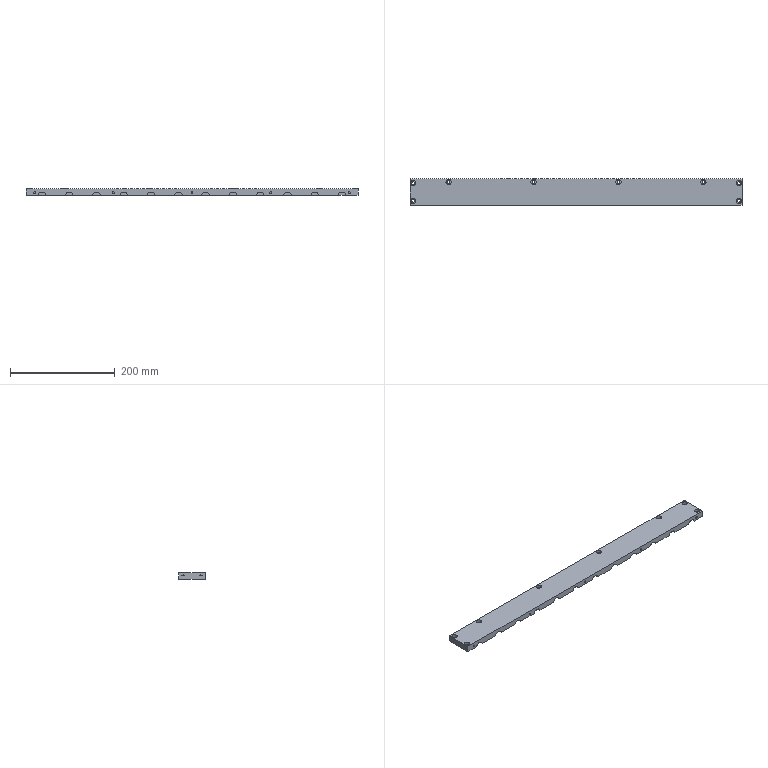Part | STEP file | Shim lower plate | 1 solid | 85 faces | box 633 x 50 x 12 mm | volume 358808 mm3 | cylinder 54 | plane 31 | commonest cylinder face diameters 5.5 x16 10 x16 16.5 x12 3.3 x10